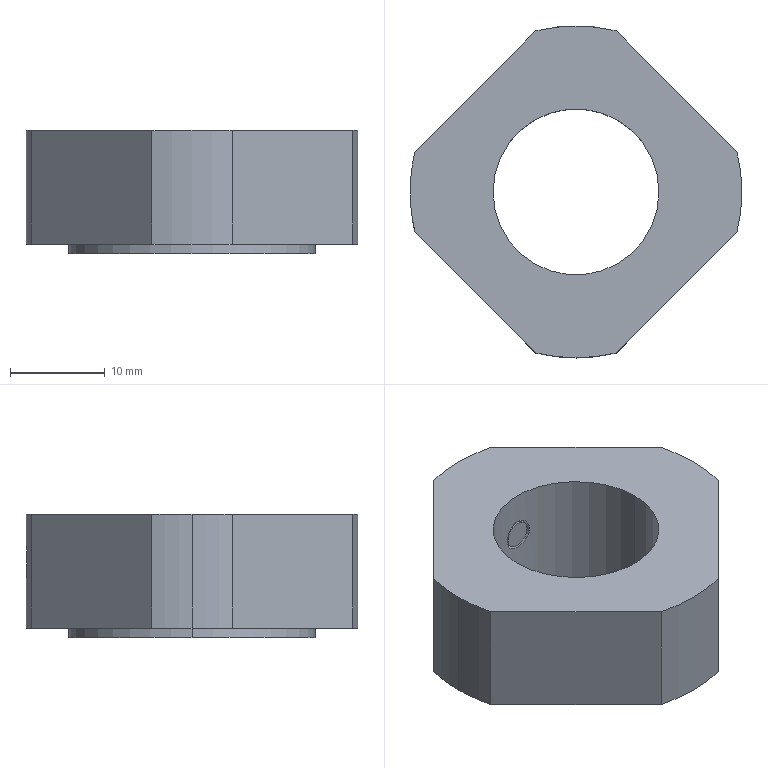Part | STEP file | Mirror BNG20 | 3 solids | 46 faces | box 35 x 35 x 13 mm | volume 7455 mm3 | plane 23 | cylinder 15 | cone 8 | commonest cylinder face diameters 35 x5 3 x2 3.3 x2 4 x2 17.5 x2 26 x2
STEP:
#1=CARTESIAN_POINT('',(-1.65,8.593,-5.));
#2=VERTEX_POINT('',#1);
#3=CARTESIAN_POINT('',(1.65,8.593,-5.));
#4=VERTEX_POINT('',#3);
#5=CARTESIAN_POINT('',(-1.65,8.593,-5.));
#6=CARTESIAN_POINT('',(-1.65,8.593,-5.109));
#7=CARTESIAN_POINT('',(-1.639,8.595,-5.217));
#8=CARTESIAN_POINT('',(-1.597,8.603,-5.428));
#9=CARTESIAN_POINT('',(-1.565,8.609,-5.533));
#10=CARTESIAN_POINT('',(-1.482,8.624,-5.733));
#11=CARTESIAN_POINT('',(-1.432,8.632,-5.827));
#12=CARTESIAN_POINT('',(-1.312,8.651,-6.006));
#13=CARTESIAN_POINT('',(-1.242,8.662,-6.091));
#14=CARTESIAN_POINT('',(-1.015,8.692,-6.319));
#15=CARTESIAN_POINT('',(-0.8309,8.713,-6.442));
#16=CARTESIAN_POINT('',(-0.4339,8.741,-6.606));
#17=CARTESIAN_POINT('',(-0.2164,8.75,-6.65));
#18=CARTESIAN_POINT('',(0.1073,8.75,-6.65));
#19=CARTESIAN_POINT('',(0.2169,8.748,-6.639));
#20=CARTESIAN_POINT('',(0.4287,8.74,-6.597));
#21=CARTESIAN_POINT('',(0.5317,8.734,-6.566));
#22=CARTESIAN_POINT('',(0.8318,8.713,-6.441));
#23=CARTESIAN_POINT('',(1.013,8.693,-6.32));
#24=CARTESIAN_POINT('',(1.244,8.662,-6.09));
#25=CARTESIAN_POINT('',(1.312,8.651,-6.007));
#26=CARTESIAN_POINT('',(1.431,8.632,-5.828));
#27=CARTESIAN_POINT('',(1.483,8.624,-5.732));
#28=CARTESIAN_POINT('',(1.566,8.609,-5.532));
#29=CARTESIAN_POINT('',(1.597,8.603,-5.429));
#30=CARTESIAN_POINT('',(1.639,8.595,-5.217));
#31=CARTESIAN_POINT('',(1.65,8.593,-5.108));
#32=CARTESIAN_POINT('',(1.65,8.593,-5.));
#33=B_SPLINE_CURVE_WITH_KNOTS('',3,(#5,#6,#7,#8,#9,#10,#11,#12,#13,#14,#15,#16,#17,#18,#19,#20,#21,#22,#23,#24,#25,#26,#27,#28,#29,#30,#31,#32),.UNSPECIFIED.,.F.,.F.,(4,2,2,2,2,2,2,2,2,2,2,2,2,4),(0.,0.0003231,0.0006463,0.0009694,0.001293,0.001939,0.002585,0.002908,0.003231,0.003878,0.004201,0.004524,0.004847,0.00517),.UNSPECIFIED.);
#34=EDGE_CURVE('',#2,#4,#33,.T.);
#35=ORIENTED_EDGE('',*,*,#34,.T.);
#36=CARTESIAN_POINT('',(1.65,17.422,-5.));
#37=VERTEX_POINT('',#36);
#38=CARTESIAN_POINT('',(1.65,17.5,-5.));
#39=DIRECTION('',(0.,1.,0.));
#40=VECTOR('',#39,1000.);
#41=LINE('',#38,#40);
#42=EDGE_CURVE('',#4,#37,#41,.T.);
#43=ORIENTED_EDGE('',*,*,#42,.T.);
#44=CARTESIAN_POINT('',(-1.65,17.422,-5.));
#45=VERTEX_POINT('',#44);
#46=CARTESIAN_POINT('',(1.65,17.422,-5.));
#47=CARTESIAN_POINT('',(1.65,17.422,-5.215));
#48=CARTESIAN_POINT('',(1.607,17.426,-5.433));
#49=CARTESIAN_POINT('',(1.442,17.441,-5.83));
#50=CARTESIAN_POINT('',(1.32,17.451,-6.014));
#51=CARTESIAN_POINT('',(1.092,17.466,-6.242));
#52=CARTESIAN_POINT('',(1.007,17.471,-6.312));
#53=CARTESIAN_POINT('',(0.8275,17.481,-6.432));
#54=CARTESIAN_POINT('',(0.7328,17.485,-6.482));
#55=CARTESIAN_POINT('',(0.5332,17.492,-6.565));
#56=CARTESIAN_POINT('',(0.4283,17.495,-6.597));
#57=CARTESIAN_POINT('',(0.2174,17.499,-6.639));
#58=CARTESIAN_POINT('',(0.1103,17.5,-6.65));
#59=CARTESIAN_POINT('',(-0.1077,17.5,-6.65));
#60=CARTESIAN_POINT('',(-0.2151,17.499,-6.639));
#61=CARTESIAN_POINT('',(-0.4261,17.495,-6.598));
#62=CARTESIAN_POINT('',(-0.5308,17.492,-6.566));
#63=CARTESIAN_POINT('',(-0.7308,17.485,-6.483));
#64=CARTESIAN_POINT('',(-0.8255,17.481,-6.433));
#65=CARTESIAN_POINT('',(-1.005,17.471,-6.313));
#66=CARTESIAN_POINT('',(-1.09,17.466,-6.244));
#67=CARTESIAN_POINT('',(-1.318,17.451,-6.016));
#68=CARTESIAN_POINT('',(-1.441,17.441,-5.832));
#69=CARTESIAN_POINT('',(-1.606,17.426,-5.435));
#70=CARTESIAN_POINT('',(-1.65,17.422,-5.218));
#71=CARTESIAN_POINT('',(-1.65,17.422,-5.));
#72=B_SPLINE_CURVE_WITH_KNOTS('',3,(#46,#47,#48,#49,#50,#51,#52,#53,#54,#55,#56,#57,#58,#59,#60,#61,#62,#63,#64,#65,#66,#67,#68,#69,#70,#71),.UNSPECIFIED.,.F.,.F.,(4,2,2,2,2,2,2,2,2,2,2,2,4),(0.005162,0.005807,0.006452,0.006774,0.007097,0.007419,0.007742,0.008064,0.008387,0.008709,0.009032,0.009677,0.01032),.UNSPECIFIED.);
#73=EDGE_CURVE('',#37,#45,#72,.T.);
#74=ORIENTED_EDGE('',*,*,#73,.T.);
#75=CARTESIAN_POINT('',(-1.65,17.5,-5.));
#76=DIRECTION('',(0.,1.,0.));
#77=VECTOR('',#76,1000.);
#78=LINE('',#75,#77);
#79=EDGE_CURVE('',#2,#45,#78,.T.);
#80=ORIENTED_EDGE('',*,*,#79,.F.);
#81=EDGE_LOOP('',(#35,#43,#74,#80));
#82=FACE_OUTER_BOUND('',#81,.T.);
#83=CARTESIAN_POINT('',(0.,17.5,-5.));
#84=DIRECTION('',(0.,1.,0.));
#85=DIRECTION('',(-1.,0.,0.));
#86=AXIS2_PLACEMENT_3D('',#83,#84,#85);
#87=CYLINDRICAL_SURFACE('',#86,1.65);
#88=ADVANCED_FACE('',(#82),#87,.F.);
#89=ORIENTED_EDGE('',*,*,#34,.F.);
#90=CARTESIAN_POINT('',(1.65,8.593,-5.));
#91=CARTESIAN_POINT('',(1.65,8.593,-4.784));
#92=CARTESIAN_POINT('',(1.607,8.602,-4.567));
#93=CARTESIAN_POINT('',(1.442,8.631,-4.17));
#94=CARTESIAN_POINT('',(1.319,8.651,-3.986));
#95=CARTESIAN_POINT('',(1.091,8.682,-3.758));
#96=CARTESIAN_POINT('',(1.007,8.692,-3.688));
#97=CARTESIAN_POINT('',(0.8281,8.711,-3.569));
#98=CARTESIAN_POINT('',(0.7335,8.72,-3.518));
#99=CARTESIAN_POINT('',(0.4333,8.742,-3.393));
#100=CARTESIAN_POINT('',(0.2188,8.75,-3.35));
#101=CARTESIAN_POINT('',(-0.1081,8.75,-3.35));
#102=CARTESIAN_POINT('',(-0.2154,8.748,-3.361));
#103=CARTESIAN_POINT('',(-0.4268,8.74,-3.403));
#104=CARTESIAN_POINT('',(-0.5319,8.734,-3.434));
#105=CARTESIAN_POINT('',(-0.7313,8.72,-3.517));
#106=CARTESIAN_POINT('',(-0.826,8.711,-3.568));
#107=CARTESIAN_POINT('',(-1.006,8.692,-3.687));
#108=CARTESIAN_POINT('',(-1.09,8.682,-3.757));
#109=CARTESIAN_POINT('',(-1.318,8.652,-3.984));
#110=CARTESIAN_POINT('',(-1.441,8.631,-4.168));
#111=CARTESIAN_POINT('',(-1.606,8.602,-4.565));
#112=CARTESIAN_POINT('',(-1.65,8.593,-4.781));
#113=CARTESIAN_POINT('',(-1.65,8.593,-5.));
#114=B_SPLINE_CURVE_WITH_KNOTS('',3,(#90,#91,#92,#93,#94,#95,#96,#97,#98,#99,#100,#101,#102,#103,#104,#105,#106,#107,#108,#109,#110,#111,#112,#113),.UNSPECIFIED.,.F.,.F.,(4,2,2,2,2,2,2,2,2,2,2,4),(0.00517,0.005816,0.006462,0.006786,0.007109,0.007755,0.008078,0.008401,0.008724,0.009047,0.009693,0.01034),.UNSPECIFIED.);
#115=EDGE_CURVE('',#4,#2,#114,.T.);
#116=ORIENTED_EDGE('',*,*,#115,.F.);
#117=EDGE_LOOP('',(#89,#116));
#118=FACE_BOUND('',#117,.T.);
#119=CARTESIAN_POINT('',(-8.75,0.,-13.));
#120=VERTEX_POINT('',#119);
#121=CARTESIAN_POINT('',(8.75,0.,-13.));
#122=VERTEX_POINT('',#121);
#123=CARTESIAN_POINT('',(0.,0.,-13.));
#124=DIRECTION('',(0.,0.,-1.));
#125=DIRECTION('',(-1.,0.,0.));
#126=AXIS2_PLACEMENT_3D('',#123,#124,#125);
#127=CIRCLE('',#126,8.75);
#128=EDGE_CURVE('',#120,#122,#127,.T.);
#129=ORIENTED_EDGE('',*,*,#128,.T.);
#130=CARTESIAN_POINT('',(8.75,0.,0.));
#131=VERTEX_POINT('',#130);
#132=CARTESIAN_POINT('',(8.75,0.,0.));
#133=DIRECTION('',(0.,0.,1.));
#134=VECTOR('',#133,1000.);
#135=LINE('',#132,#134);
#136=EDGE_CURVE('',#122,#131,#135,.T.);
#137=ORIENTED_EDGE('',*,*,#136,.T.);
#138=CARTESIAN_POINT('',(-8.75,0.,0.));
#139=VERTEX_POINT('',#138);
#140=CARTESIAN_POINT('',(0.,0.,0.));
#141=DIRECTION('',(0.,0.,-1.));
#142=DIRECTION('',(-1.,0.,0.));
#143=AXIS2_PLACEMENT_3D('',#140,#141,#142);
#144=CIRCLE('',#143,8.75);
#145=EDGE_CURVE('',#139,#131,#144,.T.);
#146=ORIENTED_EDGE('',*,*,#145,.F.);
#147=CARTESIAN_POINT('',(-8.75,0.,0.));
#148=DIRECTION('',(0.,0.,1.));
#149=VECTOR('',#148,1000.);
#150=LINE('',#147,#149);
#151=EDGE_CURVE('',#120,#139,#150,.T.);
#152=ORIENTED_EDGE('',*,*,#151,.F.);
#153=EDGE_LOOP('',(#129,#137,#146,#152));
#154=FACE_OUTER_BOUND('',#153,.T.);
#155=CARTESIAN_POINT('',(0.,0.,0.));
#156=DIRECTION('',(0.,0.,1.));
#157=DIRECTION('',(-1.,0.,0.));
#158=AXIS2_PLACEMENT_3D('',#155,#156,#157);
#159=CYLINDRICAL_SURFACE('',#158,8.75);
#160=ADVANCED_FACE('',(#118,#154),#159,.F.);
#161=CARTESIAN_POINT('',(13.,0.,-13.));
#162=VERTEX_POINT('',#161);
#163=CARTESIAN_POINT('',(-13.,0.,-13.));
#164=VERTEX_POINT('',#163);
#165=CARTESIAN_POINT('',(0.,0.,-13.));
#166=DIRECTION('',(0.,0.,-1.));
#167=DIRECTION('',(-1.,0.,0.));
#168=AXIS2_PLACEMENT_3D('',#165,#166,#167);
#169=CIRCLE('',#168,13.);
#170=EDGE_CURVE('',#162,#164,#169,.T.);
#171=ORIENTED_EDGE('',*,*,#170,.F.);
#172=CARTESIAN_POINT('',(13.,0.,-12.));
#173=VERTEX_POINT('',#172);
#174=CARTESIAN_POINT('',(13.,0.,0.));
#175=DIRECTION('',(0.,0.,1.));
#176=VECTOR('',#175,1000.);
#177=LINE('',#174,#176);
#178=EDGE_CURVE('',#162,#173,#177,.T.);
#179=ORIENTED_EDGE('',*,*,#178,.T.);
#180=CARTESIAN_POINT('',(-13.,0.,-12.));
#181=VERTEX_POINT('',#180);
#182=CARTESIAN_POINT('',(0.,0.,-12.));
#183=DIRECTION('',(0.,0.,-1.));
#184=DIRECTION('',(-1.,0.,0.));
#185=AXIS2_PLACEMENT_3D('',#182,#183,#184);
#186=CIRCLE('',#185,13.);
#187=EDGE_CURVE('',#173,#181,#186,.T.);
#188=ORIENTED_EDGE('',*,*,#187,.T.);
#189=CARTESIAN_POINT('',(-13.,0.,0.));
#190=DIRECTION('',(0.,0.,1.));
#191=VECTOR('',#190,1000.);
#192=LINE('',#189,#191);
#193=EDGE_CURVE('',#164,#181,#192,.T.);
#194=ORIENTED_EDGE('',*,*,#193,.F.);
#195=EDGE_LOOP('',(#171,#179,#188,#194));
#196=FACE_OUTER_BOUND('',#195,.T.);
#197=CARTESIAN_POINT('',(0.,0.,0.));
#198=DIRECTION('',(0.,0.,1.));
#199=DIRECTION('',(-1.,0.,0.));
#200=AXIS2_PLACEMENT_3D('',#197,#198,#199);
#201=CYLINDRICAL_SURFACE('',#200,13.);
#202=ADVANCED_FACE('',(#196),#201,.T.);
#203=CARTESIAN_POINT('',(-17.5,0.,-12.));
#204=VERTEX_POINT('',#203);
#205=CARTESIAN_POINT('',(-16.98,4.233,-12.));
#206=VERTEX_POINT('',#205);
#207=CARTESIAN_POINT('',(0.,0.,-12.));
#208=DIRECTION('',(0.,0.,-1.));
#209=DIRECTION('',(-1.,0.,0.));
#210=AXIS2_PLACEMENT_3D('',#207,#208,#209);
#211=CIRCLE('',#210,17.5);
#212=EDGE_CURVE('',#204,#206,#211,.T.);
#213=ORIENTED_EDGE('',*,*,#212,.F.);
#214=CARTESIAN_POINT('',(-17.5,0.,0.));
#215=VERTEX_POINT('',#214);
#216=CARTESIAN_POINT('',(-17.5,0.,0.));
#217=DIRECTION('',(0.,0.,1.));
#218=VECTOR('',#217,1000.);
#219=LINE('',#216,#218);
#220=EDGE_CURVE('',#204,#215,#219,.T.);
#221=ORIENTED_EDGE('',*,*,#220,.T.);
#222=CARTESIAN_POINT('',(-16.98,4.233,0.));
#223=VERTEX_POINT('',#222);
#224=CARTESIAN_POINT('',(0.,0.,0.));
#225=DIRECTION('',(0.,0.,-1.));
#226=DIRECTION('',(-1.,0.,0.));
#227=AXIS2_PLACEMENT_3D('',#224,#225,#226);
#228=CIRCLE('',#227,17.5);
#229=EDGE_CURVE('',#215,#223,#228,.T.);
#230=ORIENTED_EDGE('',*,*,#229,.T.);
#231=CARTESIAN_POINT('',(-16.98,4.233,-13.));
#232=DIRECTION('',(0.,0.,1.));
#233=VECTOR('',#232,1000.);
#234=LINE('',#231,#233);
#235=EDGE_CURVE('',#206,#223,#234,.T.);
#236=ORIENTED_EDGE('',*,*,#235,.F.);
#237=EDGE_LOOP('',(#213,#221,#230,#236));
#238=FACE_OUTER_BOUND('',#237,.T.);
#239=CARTESIAN_POINT('',(0.,0.,0.));
#240=DIRECTION('',(0.,0.,1.));
#241=DIRECTION('',(-1.,0.,0.));
#242=AXIS2_PLACEMENT_3D('',#239,#240,#241);
#243=CYLINDRICAL_SURFACE('',#242,17.5);
#244=ADVANCED_FACE('',(#238),#243,.T.);
#245=ORIENTED_EDGE('',*,*,#145,.T.);
#246=CARTESIAN_POINT('',(0.,0.,0.));
#247=DIRECTION('',(0.,0.,-1.));
#248=DIRECTION('',(-1.,0.,0.));
#249=AXIS2_PLACEMENT_3D('',#246,#247,#248);
#250=CIRCLE('',#249,8.75);
#251=EDGE_CURVE('',#131,#139,#250,.T.);
#252=ORIENTED_EDGE('',*,*,#251,.T.);
#253=EDGE_LOOP('',(#245,#252));
#254=FACE_BOUND('',#253,.T.);
#255=CARTESIAN_POINT('',(4.233,16.98,0.));
#256=VERTEX_POINT('',#255);
#257=CARTESIAN_POINT('',(16.98,4.233,0.));
#258=VERTEX_POINT('',#257);
#259=CARTESIAN_POINT('',(4.233,16.98,0.));
#260=DIRECTION('',(0.7071,-0.7071,0.));
#261=VECTOR('',#260,1000.);
#262=LINE('',#259,#261);
#263=EDGE_CURVE('',#256,#258,#262,.T.);
#264=ORIENTED_EDGE('',*,*,#263,.F.);
#265=CARTESIAN_POINT('',(-4.233,16.98,0.));
#266=VERTEX_POINT('',#265);
#267=CARTESIAN_POINT('',(0.,0.,0.));
#268=DIRECTION('',(0.,0.,-1.));
#269=DIRECTION('',(-1.,0.,0.));
#270=AXIS2_PLACEMENT_3D('',#267,#268,#269);
#271=CIRCLE('',#270,17.5);
#272=EDGE_CURVE('',#266,#256,#271,.T.);
#273=ORIENTED_EDGE('',*,*,#272,.F.);
#274=CARTESIAN_POINT('',(-16.98,4.233,0.));
#275=DIRECTION('',(0.7071,0.7071,0.));
#276=VECTOR('',#275,1000.);
#277=LINE('',#274,#276);
#278=EDGE_CURVE('',#223,#266,#277,.T.);
#279=ORIENTED_EDGE('',*,*,#278,.F.);
#280=ORIENTED_EDGE('',*,*,#229,.F.);
#281=CARTESIAN_POINT('',(-16.98,-4.233,0.));
#282=VERTEX_POINT('',#281);
#283=CARTESIAN_POINT('',(0.,0.,0.));
#284=DIRECTION('',(0.,0.,-1.));
#285=DIRECTION('',(-1.,0.,0.));
#286=AXIS2_PLACEMENT_3D('',#283,#284,#285);
#287=CIRCLE('',#286,17.5);
#288=EDGE_CURVE('',#282,#215,#287,.T.);
#289=ORIENTED_EDGE('',*,*,#288,.F.);
#290=CARTESIAN_POINT('',(-4.233,-16.98,0.));
#291=VERTEX_POINT('',#290);
#292=CARTESIAN_POINT('',(-16.98,-4.233,0.));
#293=DIRECTION('',(-0.7071,0.7071,0.));
#294=VECTOR('',#293,1000.);
#295=LINE('',#292,#294);
#296=EDGE_CURVE('',#291,#282,#295,.T.);
#297=ORIENTED_EDGE('',*,*,#296,.F.);
#298=CARTESIAN_POINT('',(4.233,-16.98,0.));
#299=VERTEX_POINT('',#298);
#300=CARTESIAN_POINT('',(0.,0.,0.));
#301=DIRECTION('',(0.,0.,-1.));
#302=DIRECTION('',(-1.,0.,0.));
#303=AXIS2_PLACEMENT_3D('',#300,#301,#302);
#304=CIRCLE('',#303,17.5);
#305=EDGE_CURVE('',#299,#291,#304,.T.);
#306=ORIENTED_EDGE('',*,*,#305,.F.);
#307=CARTESIAN_POINT('',(16.98,-4.233,0.));
#308=VERTEX_POINT('',#307);
#309=CARTESIAN_POINT('',(16.98,-4.233,0.));
#310=DIRECTION('',(-0.7071,-0.7071,0.));
#311=VECTOR('',#310,1000.);
#312=LINE('',#309,#311);
#313=EDGE_CURVE('',#308,#299,#312,.T.);
#314=ORIENTED_EDGE('',*,*,#313,.F.);
#315=CARTESIAN_POINT('',(0.,0.,0.));
#316=DIRECTION('',(0.,0.,-1.));
#317=DIRECTION('',(-1.,0.,0.));
#318=AXIS2_PLACEMENT_3D('',#315,#316,#317);
#319=CIRCLE('',#318,17.5);
#320=EDGE_CURVE('',#258,#308,#319,.T.);
#321=ORIENTED_EDGE('',*,*,#320,.F.);
#322=EDGE_LOOP('',(#264,#273,#279,#280,#289,#297,#306,#314,#321));
#323=FACE_OUTER_BOUND('',#322,.T.);
#324=CARTESIAN_POINT('',(0.,0.,0.));
#325=DIRECTION('',(0.,0.,-1.));
#326=DIRECTION('',(1.,0.,0.));
#327=AXIS2_PLACEMENT_3D('',#324,#325,#326);
#328=PLANE('',#327);
#329=ADVANCED_FACE('',(#254,#323),#328,.F.);
#330=CARTESIAN_POINT('',(16.98,4.233,-12.));
#331=VERTEX_POINT('',#330);
#332=CARTESIAN_POINT('',(16.98,4.233,-13.));
#333=DIRECTION('',(0.,0.,1.));
#334=VECTOR('',#333,1000.);
#335=LINE('',#332,#334);
#336=EDGE_CURVE('',#331,#258,#335,.T.);
#337=ORIENTED_EDGE('',*,*,#336,.T.);
#338=ORIENTED_EDGE('',*,*,#320,.T.);
#339=CARTESIAN_POINT('',(16.98,-4.233,-12.));
#340=VERTEX_POINT('',#339);
#341=CARTESIAN_POINT('',(16.98,-4.233,-13.));
#342=DIRECTION('',(0.,0.,1.));
#343=VECTOR('',#342,1000.);
#344=LINE('',#341,#343);
#345=EDGE_CURVE('',#340,#308,#344,.T.);
#346=ORIENTED_EDGE('',*,*,#345,.F.);
#347=CARTESIAN_POINT('',(0.,0.,-12.));
#348=DIRECTION('',(0.,0.,-1.));
#349=DIRECTION('',(-1.,0.,0.));
#350=AXIS2_PLACEMENT_3D('',#347,#348,#349);
#351=CIRCLE('',#350,17.5);
#352=EDGE_CURVE('',#331,#340,#351,.T.);
#353=ORIENTED_EDGE('',*,*,#352,.F.);
#354=EDGE_LOOP('',(#337,#338,#346,#353));
#355=FACE_OUTER_BOUND('',#354,.T.);
#356=CARTESIAN_POINT('',(0.,0.,0.));
#357=DIRECTION('',(0.,0.,1.));
#358=DIRECTION('',(-1.,0.,0.));
#359=AXIS2_PLACEMENT_3D('',#356,#357,#358);
#360=CYLINDRICAL_SURFACE('',#359,17.5);
#361=ADVANCED_FACE('',(#355),#360,.T.);
#362=CARTESIAN_POINT('',(-1.65,17.422,-5.));
#363=CARTESIAN_POINT('',(-1.65,17.422,-4.891));
#364=CARTESIAN_POINT('',(-1.639,17.423,-4.784));
#365=CARTESIAN_POINT('',(-1.597,17.427,-4.573));
#366=CARTESIAN_POINT('',(-1.566,17.43,-4.468));
#367=CARTESIAN_POINT('',(-1.483,17.437,-4.268));
#368=CARTESIAN_POINT('',(-1.432,17.441,-4.173));
#369=CARTESIAN_POINT('',(-1.312,17.451,-3.994));
#370=CARTESIAN_POINT('',(-1.243,17.456,-3.909));
#371=CARTESIAN_POINT('',(-1.014,17.471,-3.681));
#372=CARTESIAN_POINT('',(-0.8303,17.481,-3.558));
#373=CARTESIAN_POINT('',(-0.4332,17.496,-3.393));
#374=CARTESIAN_POINT('',(-0.216,17.5,-3.35));
#375=CARTESIAN_POINT('',(0.1071,17.5,-3.35));
#376=CARTESIAN_POINT('',(0.2165,17.499,-3.361));
#377=CARTESIAN_POINT('',(0.4281,17.495,-3.403));
#378=CARTESIAN_POINT('',(0.531,17.492,-3.434));
#379=CARTESIAN_POINT('',(0.7309,17.485,-3.517));
#380=CARTESIAN_POINT('',(0.8274,17.481,-3.568));
#381=CARTESIAN_POINT('',(1.006,17.471,-3.688));
#382=CARTESIAN_POINT('',(1.089,17.466,-3.756));
#383=CARTESIAN_POINT('',(1.244,17.456,-3.91));
#384=CARTESIAN_POINT('',(1.312,17.451,-3.993));
#385=CARTESIAN_POINT('',(1.431,17.441,-4.172));
#386=CARTESIAN_POINT('',(1.483,17.437,-4.269));
#387=CARTESIAN_POINT('',(1.566,17.43,-4.468));
#388=CARTESIAN_POINT('',(1.597,17.427,-4.571));
#389=CARTESIAN_POINT('',(1.639,17.423,-4.783));
#390=CARTESIAN_POINT('',(1.65,17.422,-4.892));
#391=CARTESIAN_POINT('',(1.65,17.422,-5.));
#392=B_SPLINE_CURVE_WITH_KNOTS('',3,(#362,#363,#364,#365,#366,#367,#368,#369,#370,#371,#372,#373,#374,#375,#376,#377,#378,#379,#380,#381,#382,#383,#384,#385,#386,#387,#388,#389,#390,#391),.UNSPECIFIED.,.F.,.F.,(4,2,2,2,2,2,2,2,2,2,2,2,2,2,4),(0.,0.0003226,0.0006452,0.0009678,0.00129,0.001936,0.002581,0.002903,0.003226,0.003549,0.003871,0.004194,0.004516,0.004839,0.005162),.UNSPECIFIED.);
#393=EDGE_CURVE('',#45,#37,#392,.T.);
#394=ORIENTED_EDGE('',*,*,#393,.F.);
#395=ORIENTED_EDGE('',*,*,#73,.F.);
#396=EDGE_LOOP('',(#394,#395));
#397=FACE_BOUND('',#396,.T.);
#398=CARTESIAN_POINT('',(4.233,16.98,-12.));
#399=VERTEX_POINT('',#398);
#400=CARTESIAN_POINT('',(4.233,16.98,-13.));
#401=DIRECTION('',(0.,0.,1.));
#402=VECTOR('',#401,1000.);
#403=LINE('',#400,#402);
#404=EDGE_CURVE('',#399,#256,#403,.T.);
#405=ORIENTED_EDGE('',*,*,#404,.F.);
#406=CARTESIAN_POINT('',(-4.233,16.98,-12.));
#407=VERTEX_POINT('',#406);
#408=CARTESIAN_POINT('',(0.,0.,-12.));
#409=DIRECTION('',(0.,0.,-1.));
#410=DIRECTION('',(-1.,0.,0.));
#411=AXIS2_PLACEMENT_3D('',#408,#409,#410);
#412=CIRCLE('',#411,17.5);
#413=EDGE_CURVE('',#407,#399,#412,.T.);
#414=ORIENTED_EDGE('',*,*,#413,.F.);
#415=CARTESIAN_POINT('',(-4.233,16.98,-13.));
#416=DIRECTION('',(0.,0.,1.));
#417=VECTOR('',#416,1000.);
#418=LINE('',#415,#417);
#419=EDGE_CURVE('',#407,#266,#418,.T.);
#420=ORIENTED_EDGE('',*,*,#419,.T.);
#421=ORIENTED_EDGE('',*,*,#272,.T.);
#422=EDGE_LOOP('',(#405,#414,#420,#421));
#423=FACE_OUTER_BOUND('',#422,.T.);
#424=CARTESIAN_POINT('',(0.,0.,0.));
#425=DIRECTION('',(0.,0.,1.));
#426=DIRECTION('',(-1.,0.,0.));
#427=AXIS2_PLACEMENT_3D('',#424,#425,#426);
#428=CYLINDRICAL_SURFACE('',#427,17.5);
#429=ADVANCED_FACE('',(#397,#423),#428,.T.);
#430=CARTESIAN_POINT('',(0.,0.,-12.));
#431=DIRECTION('',(0.,0.,-1.));
#432=DIRECTION('',(-1.,0.,0.));
#433=AXIS2_PLACEMENT_3D('',#430,#431,#432);
#434=CIRCLE('',#433,13.);
#435=EDGE_CURVE('',#181,#173,#434,.T.);
#436=ORIENTED_EDGE('',*,*,#435,.F.);
#437=ORIENTED_EDGE('',*,*,#187,.F.);
#438=EDGE_LOOP('',(#436,#437));
#439=FACE_BOUND('',#438,.T.);
#440=CARTESIAN_POINT('',(1.857,19.357,-12.));
#441=DIRECTION('',(0.7071,-0.7071,0.));
#442=VECTOR('',#441,1000.);
#443=LINE('',#440,#442);
#444=EDGE_CURVE('',#399,#331,#443,.T.);
#445=ORIENTED_EDGE('',*,*,#444,.T.);
#446=ORIENTED_EDGE('',*,*,#352,.T.);
#447=CARTESIAN_POINT('',(4.233,-16.98,-12.));
#448=VERTEX_POINT('',#447);
#449=CARTESIAN_POINT('',(19.357,-1.857,-12.));
#450=DIRECTION('',(-0.7071,-0.7071,0.));
#451=VECTOR('',#450,1000.);
#452=LINE('',#449,#451);
#453=EDGE_CURVE('',#340,#448,#452,.T.);
#454=ORIENTED_EDGE('',*,*,#453,.T.);
#455=CARTESIAN_POINT('',(-4.233,-16.98,-12.));
#456=VERTEX_POINT('',#455);
#457=CARTESIAN_POINT('',(0.,0.,-12.));
#458=DIRECTION('',(0.,0.,-1.));
#459=DIRECTION('',(-1.,0.,0.));
#460=AXIS2_PLACEMENT_3D('',#457,#458,#459);
#461=CIRCLE('',#460,17.5);
#462=EDGE_CURVE('',#448,#456,#461,.T.);
#463=ORIENTED_EDGE('',*,*,#462,.T.);
#464=CARTESIAN_POINT('',(-16.98,-4.233,-12.));
#465=VERTEX_POINT('',#464);
#466=CARTESIAN_POINT('',(-19.357,-1.857,-12.));
#467=DIRECTION('',(-0.7071,0.7071,0.));
#468=VECTOR('',#467,1000.);
#469=LINE('',#466,#468);
#470=EDGE_CURVE('',#456,#465,#469,.T.);
#471=ORIENTED_EDGE('',*,*,#470,.T.);
#472=CARTESIAN_POINT('',(0.,0.,-12.));
#473=DIRECTION('',(0.,0.,-1.));
#474=DIRECTION('',(-1.,0.,0.));
#475=AXIS2_PLACEMENT_3D('',#472,#473,#474);
#476=CIRCLE('',#475,17.5);
#477=EDGE_CURVE('',#465,#204,#476,.T.);
#478=ORIENTED_EDGE('',*,*,#477,.T.);
#479=ORIENTED_EDGE('',*,*,#212,.T.);
#480=CARTESIAN_POINT('',(-1.857,19.357,-12.));
#481=DIRECTION('',(0.7071,0.7071,0.));
#482=VECTOR('',#481,1000.);
#483=LINE('',#480,#482);
#484=EDGE_CURVE('',#206,#407,#483,.T.);
#485=ORIENTED_EDGE('',*,*,#484,.T.);
#486=ORIENTED_EDGE('',*,*,#413,.T.);
#487=EDGE_LOOP('',(#445,#446,#454,#463,#471,#478,#479,#485,#486));
#488=FACE_OUTER_BOUND('',#487,.T.);
#489=CARTESIAN_POINT('',(0.,17.5,-12.));
#490=DIRECTION('',(0.,0.,1.));
#491=DIRECTION('',(-1.,0.,0.));
#492=AXIS2_PLACEMENT_3D('',#489,#490,#491);
#493=PLANE('',#492);
#494=ADVANCED_FACE('',(#439,#488),#493,.F.);
#495=CARTESIAN_POINT('',(4.233,-16.98,-13.));
#496=DIRECTION('',(0.,0.,1.));
#497=VECTOR('',#496,1000.);
#498=LINE('',#495,#497);
#499=EDGE_CURVE('',#448,#299,#498,.T.);
#500=ORIENTED_EDGE('',*,*,#499,.T.);
#501=ORIENTED_EDGE('',*,*,#305,.T.);
#502=CARTESIAN_POINT('',(-4.233,-16.98,-13.));
#503=DIRECTION('',(0.,0.,1.));
#504=VECTOR('',#503,1000.);
#505=LINE('',#502,#504);
#506=EDGE_CURVE('',#456,#291,#505,.T.);
#507=ORIENTED_EDGE('',*,*,#506,.F.);
#508=ORIENTED_EDGE('',*,*,#462,.F.);
#509=EDGE_LOOP('',(#500,#501,#507,#508));
#510=FACE_OUTER_BOUND('',#509,.T.);
#511=CARTESIAN_POINT('',(0.,0.,0.));
#512=DIRECTION('',(0.,0.,1.));
#513=DIRECTION('',(-1.,0.,0.));
#514=AXIS2_PLACEMENT_3D('',#511,#512,#513);
#515=CYLINDRICAL_SURFACE('',#514,17.5);
#516=ADVANCED_FACE('',(#510),#515,.T.);
#517=ORIENTED_EDGE('',*,*,#220,.F.);
#518=ORIENTED_EDGE('',*,*,#477,.F.);
#519=CARTESIAN_POINT('',(-16.98,-4.233,-13.));
#520=DIRECTION('',(0.,0.,1.));
#521=VECTOR('',#520,1000.);
#522=LINE('',#519,#521);
#523=EDGE_CURVE('',#465,#282,#522,.T.);
#524=ORIENTED_EDGE('',*,*,#523,.T.);
#525=ORIENTED_EDGE('',*,*,#288,.T.);
#526=EDGE_LOOP('',(#517,#518,#524,#525));
#527=FACE_OUTER_BOUND('',#526,.T.);
#528=CARTESIAN_POINT('',(0.,0.,0.));
#529=DIRECTION('',(0.,0.,1.));
#530=DIRECTION('',(-1.,0.,0.));
#531=AXIS2_PLACEMENT_3D('',#528,#529,#530);
#532=CYLINDRICAL_SURFACE('',#531,17.5);
#533=ADVANCED_FACE('',(#527),#532,.T.);
#534=ORIENTED_EDGE('',*,*,#178,.F.);
#535=CARTESIAN_POINT('',(0.,0.,-13.));
#536=DIRECTION('',(0.,0.,-1.));
#537=DIRECTION('',(-1.,0.,0.));
#538=AXIS2_PLACEMENT_3D('',#535,#536,#537);
#539=CIRCLE('',#538,13.);
#540=EDGE_CURVE('',#164,#162,#539,.T.);
#541=ORIENTED_EDGE('',*,*,#540,.F.);
#542=ORIENTED_EDGE('',*,*,#193,.T.);
#543=ORIENTED_EDGE('',*,*,#435,.T.);
#544=EDGE_LOOP('',(#534,#541,#542,#543));
#545=FACE_OUTER_BOUND('',#544,.T.);
#546=CARTESIAN_POINT('',(0.,0.,0.));
#547=DIRECTION('',(0.,0.,1.));
#548=DIRECTION('',(-1.,0.,0.));
#549=AXIS2_PLACEMENT_3D('',#546,#547,#548);
#550=CYLINDRICAL_SURFACE('',#549,13.);
#551=ADVANCED_FACE('',(#545),#550,.T.);
#552=ORIENTED_EDGE('',*,*,#128,.F.);
#553=CARTESIAN_POINT('',(0.,0.,-13.));
#554=DIRECTION('',(0.,0.,-1.));
#555=DIRECTION('',(-1.,0.,0.));
#556=AXIS2_PLACEMENT_3D('',#553,#554,#555);
#557=CIRCLE('',#556,8.75);
#558=EDGE_CURVE('',#122,#120,#557,.T.);
#559=ORIENTED_EDGE('',*,*,#558,.F.);
#560=EDGE_LOOP('',(#552,#559));
#561=FACE_BOUND('',#560,.T.);
#562=ORIENTED_EDGE('',*,*,#540,.T.);
#563=ORIENTED_EDGE('',*,*,#170,.T.);
#564=EDGE_LOOP('',(#562,#563));
#565=FACE_OUTER_BOUND('',#564,.T.);
#566=CARTESIAN_POINT('',(0.,13.,-13.));
#567=DIRECTION('',(0.,0.,1.));
#568=DIRECTION('',(-1.,0.,0.));
#569=AXIS2_PLACEMENT_3D('',#566,#567,#568);
#570=PLANE('',#569);
#571=ADVANCED_FACE('',(#561,#565),#570,.F.);
#572=ORIENTED_EDGE('',*,*,#136,.F.);
#573=ORIENTED_EDGE('',*,*,#558,.T.);
#574=ORIENTED_EDGE('',*,*,#151,.T.);
#575=ORIENTED_EDGE('',*,*,#251,.F.);
#576=EDGE_LOOP('',(#572,#573,#574,#575));
#577=FACE_OUTER_BOUND('',#576,.T.);
#578=CARTESIAN_POINT('',(0.,0.,0.));
#579=DIRECTION('',(0.,0.,1.));
#580=DIRECTION('',(-1.,0.,0.));
#581=AXIS2_PLACEMENT_3D('',#578,#579,#580);
#582=CYLINDRICAL_SURFACE('',#581,8.75);
#583=ADVANCED_FACE('',(#577),#582,.F.);
#584=ORIENTED_EDGE('',*,*,#470,.F.);
#585=ORIENTED_EDGE('',*,*,#506,.T.);
#586=ORIENTED_EDGE('',*,*,#296,.T.);
#587=ORIENTED_EDGE('',*,*,#523,.F.);
#588=EDGE_LOOP('',(#584,#585,#586,#587));
#589=FACE_OUTER_BOUND('',#588,.T.);
#590=CARTESIAN_POINT('',(-16.98,-4.233,-13.));
#591=DIRECTION('',(-0.7071,-0.7071,0.));
#592=DIRECTION('',(0.7071,-0.7071,0.));
#593=AXIS2_PLACEMENT_3D('',#590,#591,#592);
#594=PLANE('',#593);
#595=ADVANCED_FACE('',(#589),#594,.T.);
#596=ORIENTED_EDGE('',*,*,#484,.F.);
#597=ORIENTED_EDGE('',*,*,#235,.T.);
#598=ORIENTED_EDGE('',*,*,#278,.T.);
#599=ORIENTED_EDGE('',*,*,#419,.F.);
#600=EDGE_LOOP('',(#596,#597,#598,#599));
#601=FACE_OUTER_BOUND('',#600,.T.);
#602=CARTESIAN_POINT('',(-16.98,4.233,-13.));
#603=DIRECTION('',(-0.7071,0.7071,0.));
#604=DIRECTION('',(-0.7071,-0.7071,0.));
#605=AXIS2_PLACEMENT_3D('',#602,#603,#604);
#606=PLANE('',#605);
#607=ADVANCED_FACE('',(#601),#606,.T.);
#608=ORIENTED_EDGE('',*,*,#453,.F.);
#609=ORIENTED_EDGE('',*,*,#345,.T.);
#610=ORIENTED_EDGE('',*,*,#313,.T.);
#611=ORIENTED_EDGE('',*,*,#499,.F.);
#612=EDGE_LOOP('',(#608,#609,#610,#611));
#613=FACE_OUTER_BOUND('',#612,.T.);
#614=CARTESIAN_POINT('',(16.98,-4.233,-13.));
#615=DIRECTION('',(0.7071,-0.7071,0.));
#616=DIRECTION('',(0.7071,0.7071,0.));
#617=AXIS2_PLACEMENT_3D('',#614,#615,#616);
#618=PLANE('',#617);
#619=ADVANCED_FACE('',(#613),#618,.T.);
#620=ORIENTED_EDGE('',*,*,#444,.F.);
#621=ORIENTED_EDGE('',*,*,#404,.T.);
#622=ORIENTED_EDGE('',*,*,#263,.T.);
#623=ORIENTED_EDGE('',*,*,#336,.F.);
#624=EDGE_LOOP('',(#620,#621,#622,#623));
#625=FACE_OUTER_BOUND('',#624,.T.);
#626=CARTESIAN_POINT('',(4.233,16.98,-13.));
#627=DIRECTION('',(0.7071,0.7071,0.));
#628=DIRECTION('',(-0.7071,0.7071,0.));
#629=AXIS2_PLACEMENT_3D('',#626,#627,#628);
#630=PLANE('',#629);
#631=ADVANCED_FACE('',(#625),#630,.T.);
#632=ORIENTED_EDGE('',*,*,#42,.F.);
#633=ORIENTED_EDGE('',*,*,#115,.T.);
#634=ORIENTED_EDGE('',*,*,#79,.T.);
#635=ORIENTED_EDGE('',*,*,#393,.T.);
#636=EDGE_LOOP('',(#632,#633,#634,#635));
#637=FACE_OUTER_BOUND('',#636,.T.);
#638=CARTESIAN_POINT('',(0.,17.5,-5.));
#639=DIRECTION('',(0.,1.,0.));
#640=DIRECTION('',(-1.,0.,0.));
#641=AXIS2_PLACEMENT_3D('',#638,#639,#640);
#642=CYLINDRICAL_SURFACE('',#641,1.65);
#643=ADVANCED_FACE('',(#637),#642,.F.);
#644=CLOSED_SHELL('',(#88,#160,#202,#244,#329,#361,#429,#494,#516,#533,#551,#571,#583,#595,#607,#619,#631,#643));
#645=MANIFOLD_SOLID_BREP('',#644);
#646=CARTESIAN_POINT('',(-1.25,13.5,-5.));
#647=VERTEX_POINT('',#646);
#648=CARTESIAN_POINT('',(1.25,13.5,-5.));
#649=VERTEX_POINT('',#648);
#650=CARTESIAN_POINT('',(0.,13.5,-5.));
#651=DIRECTION('',(0.,1.,0.));
#652=DIRECTION('',(1.,0.,0.));
#653=AXIS2_PLACEMENT_3D('',#650,#651,#652);
#654=CIRCLE('',#653,1.25);
#655=EDGE_CURVE('',#647,#649,#654,.T.);
#656=ORIENTED_EDGE('',*,*,#655,.T.);
#657=CARTESIAN_POINT('',(2.,14.25,-5.));
#658=VERTEX_POINT('',#657);
#659=CARTESIAN_POINT('',(2.,14.25,-5.));
#660=DIRECTION('',(0.7071,0.7071,0.));
#661=VECTOR('',#660,1000.);
#662=LINE('',#659,#661);
#663=EDGE_CURVE('',#649,#658,#662,.T.);
#664=ORIENTED_EDGE('',*,*,#663,.T.);
#665=CARTESIAN_POINT('',(0.,14.25,-3.));
#666=VERTEX_POINT('',#665);
#667=CARTESIAN_POINT('',(0.,14.25,-5.));
#668=DIRECTION('',(0.,1.,0.));
#669=DIRECTION('',(1.,0.,0.));
#670=AXIS2_PLACEMENT_3D('',#667,#668,#669);
#671=CIRCLE('',#670,2.);
#672=EDGE_CURVE('',#666,#658,#671,.T.);
#673=ORIENTED_EDGE('',*,*,#672,.F.);
#674=CARTESIAN_POINT('',(-2.,14.25,-5.));
#675=VERTEX_POINT('',#674);
#676=CARTESIAN_POINT('',(0.,14.25,-5.));
#677=DIRECTION('',(0.,1.,0.));
#678=DIRECTION('',(1.,0.,0.));
#679=AXIS2_PLACEMENT_3D('',#676,#677,#678);
#680=CIRCLE('',#679,2.);
#681=EDGE_CURVE('',#675,#666,#680,.T.);
#682=ORIENTED_EDGE('',*,*,#681,.F.);
#683=CARTESIAN_POINT('',(-2.,14.25,-5.));
#684=DIRECTION('',(-0.7071,0.7071,0.));
#685=VECTOR('',#684,1000.);
#686=LINE('',#683,#685);
#687=EDGE_CURVE('',#647,#675,#686,.T.);
#688=ORIENTED_EDGE('',*,*,#687,.F.);
#689=EDGE_LOOP('',(#656,#664,#673,#682,#688));
#690=FACE_OUTER_BOUND('',#689,.T.);
#691=CARTESIAN_POINT('',(0.,14.25,-5.));
#692=DIRECTION('',(0.,1.,0.));
#693=DIRECTION('',(-1.,0.,0.));
#694=AXIS2_PLACEMENT_3D('',#691,#692,#693);
#695=CONICAL_SURFACE('',#694,2.,0.7854);
#696=ADVANCED_FACE('',(#690),#695,.T.);
#697=CARTESIAN_POINT('',(0.,15.423,-5.));
#698=VERTEX_POINT('',#697);
#699=CARTESIAN_POINT('',(0.,16.,-4.));
#700=VERTEX_POINT('',#699);
#701=CARTESIAN_POINT('',(0.,15.423,-5.));
#702=DIRECTION('',(0.,0.5,0.866));
#703=VECTOR('',#702,1000.);
#704=LINE('',#701,#703);
#705=EDGE_CURVE('',#698,#700,#704,.T.);
#706=ORIENTED_EDGE('',*,*,#705,.F.);
#707=CARTESIAN_POINT('',(0.,16.,-6.));
#708=VERTEX_POINT('',#707);
#709=CARTESIAN_POINT('',(0.,15.423,-5.));
#710=DIRECTION('',(0.,0.5,-0.866));
#711=VECTOR('',#710,1000.);
#712=LINE('',#709,#711);
#713=EDGE_CURVE('',#698,#708,#712,.T.);
#714=ORIENTED_EDGE('',*,*,#713,.T.);
#715=CARTESIAN_POINT('',(-0.866,16.,-5.5));
#716=VERTEX_POINT('',#715);
#717=CARTESIAN_POINT('',(0.,16.,-5.));
#718=DIRECTION('',(0.,-1.,0.));
#719=DIRECTION('',(0.,0.,1.));
#720=AXIS2_PLACEMENT_3D('',#717,#718,#719);
#721=CIRCLE('',#720,1.);
#722=EDGE_CURVE('',#716,#708,#721,.T.);
#723=ORIENTED_EDGE('',*,*,#722,.F.);
#724=CARTESIAN_POINT('',(-0.866,16.,-4.5));
#725=VERTEX_POINT('',#724);
#726=CARTESIAN_POINT('',(0.,16.,-5.));
#727=DIRECTION('',(0.,-1.,0.));
#728=DIRECTION('',(0.,0.,1.));
#729=AXIS2_PLACEMENT_3D('',#726,#727,#728);
#730=CIRCLE('',#729,1.);
#731=EDGE_CURVE('',#725,#716,#730,.T.);
#732=ORIENTED_EDGE('',*,*,#731,.F.);
#733=CARTESIAN_POINT('',(0.,16.,-5.));
#734=DIRECTION('',(0.,-1.,0.));
#735=DIRECTION('',(0.,0.,1.));
#736=AXIS2_PLACEMENT_3D('',#733,#734,#735);
#737=CIRCLE('',#736,1.);
#738=EDGE_CURVE('',#700,#725,#737,.T.);
#739=ORIENTED_EDGE('',*,*,#738,.F.);
#740=EDGE_LOOP('',(#706,#714,#723,#732,#739));
#741=FACE_OUTER_BOUND('',#740,.T.);
#742=CARTESIAN_POINT('',(0.,1015.423,-5.));
#743=DIRECTION('',(0.,1.,0.));
#744=DIRECTION('',(0.,0.,1.));
#745=AXIS2_PLACEMENT_3D('',#742,#743,#744);
#746=CONICAL_SURFACE('',#745,1732.051,1.047);
#747=ADVANCED_FACE('',(#741),#746,.F.);
#748=ORIENTED_EDGE('',*,*,#672,.T.);
#749=CARTESIAN_POINT('',(0.,14.25,-7.));
#750=VERTEX_POINT('',#749);
#751=CARTESIAN_POINT('',(0.,14.25,-5.));
#752=DIRECTION('',(0.,1.,0.));
#753=DIRECTION('',(1.,0.,0.));
#754=AXIS2_PLACEMENT_3D('',#751,#752,#753);
#755=CIRCLE('',#754,2.);
#756=EDGE_CURVE('',#658,#750,#755,.T.);
#757=ORIENTED_EDGE('',*,*,#756,.T.);
#758=CARTESIAN_POINT('',(0.,17.5,-7.));
#759=VERTEX_POINT('',#758);
#760=CARTESIAN_POINT('',(0.,17.5,-7.));
#761=DIRECTION('',(0.,1.,0.));
#762=VECTOR('',#761,1000.);
#763=LINE('',#760,#762);
#764=EDGE_CURVE('',#750,#759,#763,.T.);
#765=ORIENTED_EDGE('',*,*,#764,.T.);
#766=CARTESIAN_POINT('',(0.,17.5,-3.));
#767=VERTEX_POINT('',#766);
#768=CARTESIAN_POINT('',(0.,17.5,-5.));
#769=DIRECTION('',(0.,-1.,0.));
#770=DIRECTION('',(0.,0.,1.));
#771=AXIS2_PLACEMENT_3D('',#768,#769,#770);
#772=CIRCLE('',#771,2.);
#773=EDGE_CURVE('',#759,#767,#772,.T.);
#774=ORIENTED_EDGE('',*,*,#773,.T.);
#775=CARTESIAN_POINT('',(0.,17.5,-3.));
#776=DIRECTION('',(0.,1.,0.));
#777=VECTOR('',#776,1000.);
#778=LINE('',#775,#777);
#779=EDGE_CURVE('',#666,#767,#778,.T.);
#780=ORIENTED_EDGE('',*,*,#779,.F.);
#781=EDGE_LOOP('',(#748,#757,#765,#774,#780));
#782=FACE_OUTER_BOUND('',#781,.T.);
#783=CARTESIAN_POINT('',(0.,17.5,-5.));
#784=DIRECTION('',(0.,1.,0.));
#785=DIRECTION('',(0.,0.,1.));
#786=AXIS2_PLACEMENT_3D('',#783,#784,#785);
#787=CYLINDRICAL_SURFACE('',#786,2.);
#788=ADVANCED_FACE('',(#782),#787,.T.);
#789=CARTESIAN_POINT('',(0.,17.5,-5.));
#790=DIRECTION('',(0.,-1.,0.));
#791=DIRECTION('',(0.,0.,1.));
#792=AXIS2_PLACEMENT_3D('',#789,#790,#791);
#793=CIRCLE('',#792,2.);
#794=EDGE_CURVE('',#767,#759,#793,.T.);
#795=ORIENTED_EDGE('',*,*,#794,.F.);
#796=ORIENTED_EDGE('',*,*,#773,.F.);
#797=EDGE_LOOP('',(#795,#796));
#798=FACE_OUTER_BOUND('',#797,.T.);
#799=CARTESIAN_POINT('',(1.155,17.5,-5.));
#800=VERTEX_POINT('',#799);
#801=CARTESIAN_POINT('',(0.5774,17.5,-4.));
#802=VERTEX_POINT('',#801);
#803=CARTESIAN_POINT('',(1.155,17.5,-5.));
#804=DIRECTION('',(-0.5,0.,0.866));
#805=VECTOR('',#804,1000.);
#806=LINE('',#803,#805);
#807=EDGE_CURVE('',#800,#802,#806,.T.);
#808=ORIENTED_EDGE('',*,*,#807,.T.);
#809=CARTESIAN_POINT('',(-0.5774,17.5,-4.));
#810=VERTEX_POINT('',#809);
#811=CARTESIAN_POINT('',(0.5774,17.5,-4.));
#812=DIRECTION('',(-1.,0.,0.));
#813=VECTOR('',#812,1000.);
#814=LINE('',#811,#813);
#815=EDGE_CURVE('',#802,#810,#814,.T.);
#816=ORIENTED_EDGE('',*,*,#815,.T.);
#817=CARTESIAN_POINT('',(-1.155,17.5,-5.));
#818=VERTEX_POINT('',#817);
#819=CARTESIAN_POINT('',(-0.5774,17.5,-4.));
#820=DIRECTION('',(-0.5,0.,-0.866));
#821=VECTOR('',#820,1000.);
#822=LINE('',#819,#821);
#823=EDGE_CURVE('',#810,#818,#822,.T.);
#824=ORIENTED_EDGE('',*,*,#823,.T.);
#825=CARTESIAN_POINT('',(-0.5774,17.5,-6.));
#826=VERTEX_POINT('',#825);
#827=CARTESIAN_POINT('',(-1.155,17.5,-5.));
#828=DIRECTION('',(0.5,0.,-0.866));
#829=VECTOR('',#828,1000.);
#830=LINE('',#827,#829);
#831=EDGE_CURVE('',#818,#826,#830,.T.);
#832=ORIENTED_EDGE('',*,*,#831,.T.);
#833=CARTESIAN_POINT('',(0.5774,17.5,-6.));
#834=VERTEX_POINT('',#833);
#835=CARTESIAN_POINT('',(-0.5774,17.5,-6.));
#836=DIRECTION('',(1.,0.,0.));
#837=VECTOR('',#836,1000.);
#838=LINE('',#835,#837);
#839=EDGE_CURVE('',#826,#834,#838,.T.);
#840=ORIENTED_EDGE('',*,*,#839,.T.);
#841=CARTESIAN_POINT('',(0.5774,17.5,-6.));
#842=DIRECTION('',(0.5,0.,0.866));
#843=VECTOR('',#842,1000.);
#844=LINE('',#841,#843);
#845=EDGE_CURVE('',#834,#800,#844,.T.);
#846=ORIENTED_EDGE('',*,*,#845,.T.);
#847=EDGE_LOOP('',(#808,#816,#824,#832,#840,#846));
#848=FACE_BOUND('',#847,.T.);
#849=CARTESIAN_POINT('',(0.,17.5,-5.));
#850=DIRECTION('',(0.,-1.,0.));
#851=DIRECTION('',(0.,0.,-1.));
#852=AXIS2_PLACEMENT_3D('',#849,#850,#851);
#853=PLANE('',#852);
#854=ADVANCED_FACE('',(#798,#848),#853,.F.);
#855=ORIENTED_EDGE('',*,*,#764,.F.);
#856=CARTESIAN_POINT('',(0.,14.25,-5.));
#857=DIRECTION('',(0.,1.,0.));
#858=DIRECTION('',(1.,0.,0.));
#859=AXIS2_PLACEMENT_3D('',#856,#857,#858);
#860=CIRCLE('',#859,2.);
#861=EDGE_CURVE('',#750,#675,#860,.T.);
#862=ORIENTED_EDGE('',*,*,#861,.T.);
#863=ORIENTED_EDGE('',*,*,#681,.T.);
#864=ORIENTED_EDGE('',*,*,#779,.T.);
#865=ORIENTED_EDGE('',*,*,#794,.T.);
#866=EDGE_LOOP('',(#855,#862,#863,#864,#865));
#867=FACE_OUTER_BOUND('',#866,.T.);
#868=CARTESIAN_POINT('',(0.,17.5,-5.));
#869=DIRECTION('',(0.,1.,0.));
#870=DIRECTION('',(0.,0.,1.));
#871=AXIS2_PLACEMENT_3D('',#868,#869,#870);
#872=CYLINDRICAL_SURFACE('',#871,2.);
#873=ADVANCED_FACE('',(#867),#872,.T.);
#874=CARTESIAN_POINT('',(0.5774,16.,-6.));
#875=VERTEX_POINT('',#874);
#876=CARTESIAN_POINT('',(0.866,16.,-5.5));
#877=VERTEX_POINT('',#876);
#878=CARTESIAN_POINT('',(0.5774,16.,-6.));
#879=DIRECTION('',(0.5,0.,0.866));
#880=VECTOR('',#879,1000.);
#881=LINE('',#878,#880);
#882=EDGE_CURVE('',#875,#877,#881,.T.);
#883=ORIENTED_EDGE('',*,*,#882,.T.);
#884=CARTESIAN_POINT('',(1.155,16.,-5.));
#885=VERTEX_POINT('',#884);
#886=CARTESIAN_POINT('',(0.5774,16.,-6.));
#887=DIRECTION('',(0.5,0.,0.866));
#888=VECTOR('',#887,1000.);
#889=LINE('',#886,#888);
#890=EDGE_CURVE('',#877,#885,#889,.T.);
#891=ORIENTED_EDGE('',*,*,#890,.T.);
#892=CARTESIAN_POINT('',(1.155,16.,-5.));
#893=DIRECTION('',(0.,1.,0.));
#894=VECTOR('',#893,1000.);
#895=LINE('',#892,#894);
#896=EDGE_CURVE('',#885,#800,#895,.T.);
#897=ORIENTED_EDGE('',*,*,#896,.T.);
#898=ORIENTED_EDGE('',*,*,#845,.F.);
#899=CARTESIAN_POINT('',(0.5774,16.,-6.));
#900=DIRECTION('',(0.,1.,0.));
#901=VECTOR('',#900,1000.);
#902=LINE('',#899,#901);
#903=EDGE_CURVE('',#875,#834,#902,.T.);
#904=ORIENTED_EDGE('',*,*,#903,.F.);
#905=EDGE_LOOP('',(#883,#891,#897,#898,#904));
#906=FACE_OUTER_BOUND('',#905,.T.);
#907=CARTESIAN_POINT('',(0.5774,16.,-6.));
#908=DIRECTION('',(0.866,0.,-0.5));
#909=DIRECTION('',(0.5,0.,0.866));
#910=AXIS2_PLACEMENT_3D('',#907,#908,#909);
#911=PLANE('',#910);
#912=ADVANCED_FACE('',(#906),#911,.F.);
#913=CARTESIAN_POINT('',(-0.5774,16.,-6.));
#914=VERTEX_POINT('',#913);
#915=CARTESIAN_POINT('',(-0.5774,16.,-6.));
#916=DIRECTION('',(1.,0.,0.));
#917=VECTOR('',#916,1000.);
#918=LINE('',#915,#917);
#919=EDGE_CURVE('',#914,#708,#918,.T.);
#920=ORIENTED_EDGE('',*,*,#919,.T.);
#921=CARTESIAN_POINT('',(-0.5774,16.,-6.));
#922=DIRECTION('',(1.,0.,0.));
#923=VECTOR('',#922,1000.);
#924=LINE('',#921,#923);
#925=EDGE_CURVE('',#708,#875,#924,.T.);
#926=ORIENTED_EDGE('',*,*,#925,.T.);
#927=ORIENTED_EDGE('',*,*,#903,.T.);
#928=ORIENTED_EDGE('',*,*,#839,.F.);
#929=CARTESIAN_POINT('',(-0.5774,16.,-6.));
#930=DIRECTION('',(0.,1.,0.));
#931=VECTOR('',#930,1000.);
#932=LINE('',#929,#931);
#933=EDGE_CURVE('',#914,#826,#932,.T.);
#934=ORIENTED_EDGE('',*,*,#933,.F.);
#935=EDGE_LOOP('',(#920,#926,#927,#928,#934));
#936=FACE_OUTER_BOUND('',#935,.T.);
#937=CARTESIAN_POINT('',(-0.5774,16.,-6.));
#938=DIRECTION('',(0.,0.,-1.));
#939=DIRECTION('',(1.,0.,0.));
#940=AXIS2_PLACEMENT_3D('',#937,#938,#939);
#941=PLANE('',#940);
#942=ADVANCED_FACE('',(#936),#941,.F.);
#943=CARTESIAN_POINT('',(-1.155,16.,-5.));
#944=VERTEX_POINT('',#943);
#945=CARTESIAN_POINT('',(-1.155,16.,-5.));
#946=DIRECTION('',(0.5,0.,-0.866));
#947=VECTOR('',#946,1000.);
#948=LINE('',#945,#947);
#949=EDGE_CURVE('',#944,#716,#948,.T.);
#950=ORIENTED_EDGE('',*,*,#949,.T.);
#951=CARTESIAN_POINT('',(-1.155,16.,-5.));
#952=DIRECTION('',(0.5,0.,-0.866));
#953=VECTOR('',#952,1000.);
#954=LINE('',#951,#953);
#955=EDGE_CURVE('',#716,#914,#954,.T.);
#956=ORIENTED_EDGE('',*,*,#955,.T.);
#957=ORIENTED_EDGE('',*,*,#933,.T.);
#958=ORIENTED_EDGE('',*,*,#831,.F.);
#959=CARTESIAN_POINT('',(-1.155,16.,-5.));
#960=DIRECTION('',(0.,1.,0.));
#961=VECTOR('',#960,1000.);
#962=LINE('',#959,#961);
#963=EDGE_CURVE('',#944,#818,#962,.T.);
#964=ORIENTED_EDGE('',*,*,#963,.F.);
#965=EDGE_LOOP('',(#950,#956,#957,#958,#964));
#966=FACE_OUTER_BOUND('',#965,.T.);
#967=CARTESIAN_POINT('',(-1.155,16.,-5.));
#968=DIRECTION('',(-0.866,0.,-0.5));
#969=DIRECTION('',(0.5,0.,-0.866));
#970=AXIS2_PLACEMENT_3D('',#967,#968,#969);
#971=PLANE('',#970);
#972=ADVANCED_FACE('',(#966),#971,.F.);
#973=CARTESIAN_POINT('',(-0.5774,16.,-4.));
#974=VERTEX_POINT('',#973);
#975=CARTESIAN_POINT('',(-0.5774,16.,-4.));
#976=DIRECTION('',(-0.5,0.,-0.866));
#977=VECTOR('',#976,1000.);
#978=LINE('',#975,#977);
#979=EDGE_CURVE('',#974,#725,#978,.T.);
#980=ORIENTED_EDGE('',*,*,#979,.T.);
#981=CARTESIAN_POINT('',(-0.5774,16.,-4.));
#982=DIRECTION('',(-0.5,0.,-0.866));
#983=VECTOR('',#982,1000.);
#984=LINE('',#981,#983);
#985=EDGE_CURVE('',#725,#944,#984,.T.);
#986=ORIENTED_EDGE('',*,*,#985,.T.);
#987=ORIENTED_EDGE('',*,*,#963,.T.);
#988=ORIENTED_EDGE('',*,*,#823,.F.);
#989=CARTESIAN_POINT('',(-0.5774,16.,-4.));
#990=DIRECTION('',(0.,1.,0.));
#991=VECTOR('',#990,1000.);
#992=LINE('',#989,#991);
#993=EDGE_CURVE('',#974,#810,#992,.T.);
#994=ORIENTED_EDGE('',*,*,#993,.F.);
#995=EDGE_LOOP('',(#980,#986,#987,#988,#994));
#996=FACE_OUTER_BOUND('',#995,.T.);
#997=CARTESIAN_POINT('',(-0.5774,16.,-4.));
#998=DIRECTION('',(-0.866,0.,0.5));
#999=DIRECTION('',(-0.5,0.,-0.866));
#1000=AXIS2_PLACEMENT_3D('',#997,#998,#999);
#1001=PLANE('',#1000);
#1002=ADVANCED_FACE('',(#996),#1001,.F.);
#1003=CARTESIAN_POINT('',(0.5774,16.,-4.));
#1004=VERTEX_POINT('',#1003);
#1005=CARTESIAN_POINT('',(0.5774,16.,-4.));
#1006=DIRECTION('',(-1.,0.,0.));
#1007=VECTOR('',#1006,1000.);
#1008=LINE('',#1005,#1007);
#1009=EDGE_CURVE('',#1004,#700,#1008,.T.);
#1010=ORIENTED_EDGE('',*,*,#1009,.T.);
#1011=CARTESIAN_POINT('',(0.5774,16.,-4.));
#1012=DIRECTION('',(-1.,0.,0.));
#1013=VECTOR('',#1012,1000.);
#1014=LINE('',#1011,#1013);
#1015=EDGE_CURVE('',#700,#974,#1014,.T.);
#1016=ORIENTED_EDGE('',*,*,#1015,.T.);
#1017=ORIENTED_EDGE('',*,*,#993,.T.);
#1018=ORIENTED_EDGE('',*,*,#815,.F.);
#1019=CARTESIAN_POINT('',(0.5774,16.,-4.));
#1020=DIRECTION('',(0.,1.,0.));
#1021=VECTOR('',#1020,1000.);
#1022=LINE('',#1019,#1021);
#1023=EDGE_CURVE('',#1004,#802,#1022,.T.);
#1024=ORIENTED_EDGE('',*,*,#1023,.F.);
#1025=EDGE_LOOP('',(#1010,#1016,#1017,#1018,#1024));
#1026=FACE_OUTER_BOUND('',#1025,.T.);
#1027=CARTESIAN_POINT('',(0.5774,16.,-4.));
#1028=DIRECTION('',(0.,0.,1.));
#1029=DIRECTION('',(-1.,0.,0.));
#1030=AXIS2_PLACEMENT_3D('',#1027,#1028,#1029);
#1031=PLANE('',#1030);
#1032=ADVANCED_FACE('',(#1026),#1031,.F.);
#1033=CARTESIAN_POINT('',(0.866,16.,-4.5));
#1034=VERTEX_POINT('',#1033);
#1035=CARTESIAN_POINT('',(1.155,16.,-5.));
#1036=DIRECTION('',(-0.5,0.,0.866));
#1037=VECTOR('',#1036,1000.);
#1038=LINE('',#1035,#1037);
#1039=EDGE_CURVE('',#885,#1034,#1038,.T.);
#1040=ORIENTED_EDGE('',*,*,#1039,.T.);
#1041=CARTESIAN_POINT('',(1.155,16.,-5.));
#1042=DIRECTION('',(-0.5,0.,0.866));
#1043=VECTOR('',#1042,1000.);
#1044=LINE('',#1041,#1043);
#1045=EDGE_CURVE('',#1034,#1004,#1044,.T.);
#1046=ORIENTED_EDGE('',*,*,#1045,.T.);
#1047=ORIENTED_EDGE('',*,*,#1023,.T.);
#1048=ORIENTED_EDGE('',*,*,#807,.F.);
#1049=ORIENTED_EDGE('',*,*,#896,.F.);
#1050=EDGE_LOOP('',(#1040,#1046,#1047,#1048,#1049));
#1051=FACE_OUTER_BOUND('',#1050,.T.);
#1052=CARTESIAN_POINT('',(1.155,16.,-5.));
#1053=DIRECTION('',(0.866,0.,0.5));
#1054=DIRECTION('',(-0.5,0.,0.866));
#1055=AXIS2_PLACEMENT_3D('',#1052,#1053,#1054);
#1056=PLANE('',#1055);
#1057=ADVANCED_FACE('',(#1051),#1056,.F.);
#1058=ORIENTED_EDGE('',*,*,#955,.F.);
#1059=ORIENTED_EDGE('',*,*,#722,.T.);
#1060=ORIENTED_EDGE('',*,*,#919,.F.);
#1061=EDGE_LOOP('',(#1058,#1059,#1060));
#1062=FACE_OUTER_BOUND('',#1061,.T.);
#1063=CARTESIAN_POINT('',(0.,16.,-5.));
#1064=DIRECTION('',(0.,1.,0.));
#1065=DIRECTION('',(-1.,0.,0.));
#1066=AXIS2_PLACEMENT_3D('',#1063,#1064,#1065);
#1067=PLANE('',#1066);
#1068=ADVANCED_FACE('',(#1062),#1067,.T.);
#1069=ORIENTED_EDGE('',*,*,#925,.F.);
#1070=CARTESIAN_POINT('',(0.,16.,-5.));
#1071=DIRECTION('',(0.,-1.,0.));
#1072=DIRECTION('',(0.,0.,1.));
#1073=AXIS2_PLACEMENT_3D('',#1070,#1071,#1072);
#1074=CIRCLE('',#1073,1.);
#1075=EDGE_CURVE('',#708,#877,#1074,.T.);
#1076=ORIENTED_EDGE('',*,*,#1075,.T.);
#1077=ORIENTED_EDGE('',*,*,#882,.F.);
#1078=EDGE_LOOP('',(#1069,#1076,#1077));
#1079=FACE_OUTER_BOUND('',#1078,.T.);
#1080=CARTESIAN_POINT('',(0.,16.,-5.));
#1081=DIRECTION('',(0.,1.,0.));
#1082=DIRECTION('',(-1.,0.,0.));
#1083=AXIS2_PLACEMENT_3D('',#1080,#1081,#1082);
#1084=PLANE('',#1083);
#1085=ADVANCED_FACE('',(#1079),#1084,.T.);
#1086=ORIENTED_EDGE('',*,*,#890,.F.);
#1087=CARTESIAN_POINT('',(0.,16.,-5.));
#1088=DIRECTION('',(0.,-1.,0.));
#1089=DIRECTION('',(0.,0.,1.));
#1090=AXIS2_PLACEMENT_3D('',#1087,#1088,#1089);
#1091=CIRCLE('',#1090,1.);
#1092=EDGE_CURVE('',#877,#1034,#1091,.T.);
#1093=ORIENTED_EDGE('',*,*,#1092,.T.);
#1094=ORIENTED_EDGE('',*,*,#1039,.F.);
#1095=EDGE_LOOP('',(#1086,#1093,#1094));
#1096=FACE_OUTER_BOUND('',#1095,.T.);
#1097=CARTESIAN_POINT('',(0.,16.,-5.));
#1098=DIRECTION('',(0.,1.,0.));
#1099=DIRECTION('',(-1.,0.,0.));
#1100=AXIS2_PLACEMENT_3D('',#1097,#1098,#1099);
#1101=PLANE('',#1100);
#1102=ADVANCED_FACE('',(#1096),#1101,.T.);
#1103=ORIENTED_EDGE('',*,*,#1045,.F.);
#1104=CARTESIAN_POINT('',(0.,16.,-5.));
#1105=DIRECTION('',(0.,-1.,0.));
#1106=DIRECTION('',(0.,0.,1.));
#1107=AXIS2_PLACEMENT_3D('',#1104,#1105,#1106);
#1108=CIRCLE('',#1107,1.);
#1109=EDGE_CURVE('',#1034,#700,#1108,.T.);
#1110=ORIENTED_EDGE('',*,*,#1109,.T.);
#1111=ORIENTED_EDGE('',*,*,#1009,.F.);
#1112=EDGE_LOOP('',(#1103,#1110,#1111));
#1113=FACE_OUTER_BOUND('',#1112,.T.);
#1114=CARTESIAN_POINT('',(0.,16.,-5.));
#1115=DIRECTION('',(0.,1.,0.));
#1116=DIRECTION('',(-1.,0.,0.));
#1117=AXIS2_PLACEMENT_3D('',#1114,#1115,#1116);
#1118=PLANE('',#1117);
#1119=ADVANCED_FACE('',(#1113),#1118,.T.);
#1120=ORIENTED_EDGE('',*,*,#1015,.F.);
#1121=ORIENTED_EDGE('',*,*,#738,.T.);
#1122=ORIENTED_EDGE('',*,*,#979,.F.);
#1123=EDGE_LOOP('',(#1120,#1121,#1122));
#1124=FACE_OUTER_BOUND('',#1123,.T.);
#1125=CARTESIAN_POINT('',(0.,16.,-5.));
#1126=DIRECTION('',(0.,1.,0.));
#1127=DIRECTION('',(-1.,0.,0.));
#1128=AXIS2_PLACEMENT_3D('',#1125,#1126,#1127);
#1129=PLANE('',#1128);
#1130=ADVANCED_FACE('',(#1124),#1129,.T.);
#1131=ORIENTED_EDGE('',*,*,#985,.F.);
#1132=ORIENTED_EDGE('',*,*,#731,.T.);
#1133=ORIENTED_EDGE('',*,*,#949,.F.);
#1134=EDGE_LOOP('',(#1131,#1132,#1133));
#1135=FACE_OUTER_BOUND('',#1134,.T.);
#1136=CARTESIAN_POINT('',(0.,16.,-5.));
#1137=DIRECTION('',(0.,1.,0.));
#1138=DIRECTION('',(-1.,0.,0.));
#1139=AXIS2_PLACEMENT_3D('',#1136,#1137,#1138);
#1140=PLANE('',#1139);
#1141=ADVANCED_FACE('',(#1135),#1140,.T.);
#1142=ORIENTED_EDGE('',*,*,#713,.F.);
#1143=ORIENTED_EDGE('',*,*,#705,.T.);
#1144=ORIENTED_EDGE('',*,*,#1109,.F.);
#1145=ORIENTED_EDGE('',*,*,#1092,.F.);
#1146=ORIENTED_EDGE('',*,*,#1075,.F.);
#1147=EDGE_LOOP('',(#1142,#1143,#1144,#1145,#1146));
#1148=FACE_OUTER_BOUND('',#1147,.T.);
#1149=CARTESIAN_POINT('',(0.,1015.423,-5.));
#1150=DIRECTION('',(0.,1.,0.));
#1151=DIRECTION('',(0.,0.,1.));
#1152=AXIS2_PLACEMENT_3D('',#1149,#1150,#1151);
#1153=CONICAL_SURFACE('',#1152,1732.051,1.047);
#1154=ADVANCED_FACE('',(#1148),#1153,.F.);
#1155=ORIENTED_EDGE('',*,*,#663,.F.);
#1156=CARTESIAN_POINT('',(0.,13.5,-5.));
#1157=DIRECTION('',(0.,1.,0.));
#1158=DIRECTION('',(1.,0.,0.));
#1159=AXIS2_PLACEMENT_3D('',#1156,#1157,#1158);
#1160=CIRCLE('',#1159,1.25);
#1161=EDGE_CURVE('',#649,#647,#1160,.T.);
#1162=ORIENTED_EDGE('',*,*,#1161,.T.);
#1163=ORIENTED_EDGE('',*,*,#687,.T.);
#1164=ORIENTED_EDGE('',*,*,#861,.F.);
#1165=ORIENTED_EDGE('',*,*,#756,.F.);
#1166=EDGE_LOOP('',(#1155,#1162,#1163,#1164,#1165));
#1167=FACE_OUTER_BOUND('',#1166,.T.);
#1168=CARTESIAN_POINT('',(0.,14.25,-5.));
#1169=DIRECTION('',(0.,1.,0.));
#1170=DIRECTION('',(-1.,0.,0.));
#1171=AXIS2_PLACEMENT_3D('',#1168,#1169,#1170);
#1172=CONICAL_SURFACE('',#1171,2.,0.7854);
#1173=ADVANCED_FACE('',(#1167),#1172,.T.);
#1174=ORIENTED_EDGE('',*,*,#655,.F.);
#1175=ORIENTED_EDGE('',*,*,#1161,.F.);
#1176=EDGE_LOOP('',(#1174,#1175));
#1177=FACE_OUTER_BOUND('',#1176,.T.);
#1178=CARTESIAN_POINT('',(0.,13.5,-7.));
#1179=DIRECTION('',(0.,1.,0.));
#1180=DIRECTION('',(0.,0.,1.));
#1181=AXIS2_PLACEMENT_3D('',#1178,#1179,#1180);
#1182=PLANE('',#1181);
#1183=ADVANCED_FACE('',(#1177),#1182,.F.);
#1184=CLOSED_SHELL('',(#696,#747,#788,#854,#873,#912,#942,#972,#1002,#1032,#1057,#1068,#1085,#1102,#1119,#1130,#1141,#1154,#1173,#1183));
#1185=MANIFOLD_SOLID_BREP('',#1184);
#1186=CARTESIAN_POINT('',(0.,9.25,-6.4));
#1187=VERTEX_POINT('',#1186);
#1188=CARTESIAN_POINT('',(0.,9.25,-3.6));
#1189=VERTEX_POINT('',#1188);
#1190=CARTESIAN_POINT('',(0.,9.25,-5.));
#1191=DIRECTION('',(0.,-1.,0.));
#1192=DIRECTION('',(0.,0.,-1.));
#1193=AXIS2_PLACEMENT_3D('',#1190,#1191,#1192);
#1194=CIRCLE('',#1193,1.4);
#1195=EDGE_CURVE('',#1187,#1189,#1194,.T.);
#1196=ORIENTED_EDGE('',*,*,#1195,.T.);
#1197=CARTESIAN_POINT('',(0.,9.15,-3.5));
#1198=VERTEX_POINT('',#1197);
#1199=CARTESIAN_POINT('',(0.,9.25,-3.6));
#1200=DIRECTION('',(0.,-0.7071,0.7071));
#1201=VECTOR('',#1200,1000.);
#1202=LINE('',#1199,#1201);
#1203=EDGE_CURVE('',#1189,#1198,#1202,.T.);
#1204=ORIENTED_EDGE('',*,*,#1203,.T.);
#1205=CARTESIAN_POINT('',(0.,9.15,-6.5));
#1206=VERTEX_POINT('',#1205);
#1207=CARTESIAN_POINT('',(0.,9.15,-5.));
#1208=DIRECTION('',(0.,1.,0.));
#1209=DIRECTION('',(0.,0.,-1.));
#1210=AXIS2_PLACEMENT_3D('',#1207,#1208,#1209);
#1211=CIRCLE('',#1210,1.5);
#1212=EDGE_CURVE('',#1198,#1206,#1211,.T.);
#1213=ORIENTED_EDGE('',*,*,#1212,.T.);
#1214=CARTESIAN_POINT('',(0.,9.25,-6.4));
#1215=DIRECTION('',(0.,-0.7071,-0.7071));
#1216=VECTOR('',#1215,1000.);
#1217=LINE('',#1214,#1216);
#1218=EDGE_CURVE('',#1187,#1206,#1217,.T.);
#1219=ORIENTED_EDGE('',*,*,#1218,.F.);
#1220=EDGE_LOOP('',(#1196,#1204,#1213,#1219));
#1221=FACE_OUTER_BOUND('',#1220,.T.);
#1222=CARTESIAN_POINT('',(0.,9.25,-5.));
#1223=DIRECTION('',(0.,-1.,0.));
#1224=DIRECTION('',(0.,0.,-1.));
#1225=AXIS2_PLACEMENT_3D('',#1222,#1223,#1224);
#1226=CONICAL_SURFACE('',#1225,1.4,0.7854);
#1227=ADVANCED_FACE('',(#1221),#1226,.T.);
#1228=CARTESIAN_POINT('',(0.,8.75,-3.6));
#1229=VERTEX_POINT('',#1228);
#1230=CARTESIAN_POINT('',(0.,8.75,-6.4));
#1231=VERTEX_POINT('',#1230);
#1232=CARTESIAN_POINT('',(0.,8.75,-5.));
#1233=DIRECTION('',(0.,1.,0.));
#1234=DIRECTION('',(0.,0.,1.));
#1235=AXIS2_PLACEMENT_3D('',#1232,#1233,#1234);
#1236=CIRCLE('',#1235,1.4);
#1237=EDGE_CURVE('',#1229,#1231,#1236,.T.);
#1238=ORIENTED_EDGE('',*,*,#1237,.T.);
#1239=CARTESIAN_POINT('',(0.,8.85,-6.5));
#1240=VERTEX_POINT('',#1239);
#1241=CARTESIAN_POINT('',(0.,8.85,-6.5));
#1242=DIRECTION('',(0.,0.7071,-0.7071));
#1243=VECTOR('',#1242,1000.);
#1244=LINE('',#1241,#1243);
#1245=EDGE_CURVE('',#1231,#1240,#1244,.T.);
#1246=ORIENTED_EDGE('',*,*,#1245,.T.);
#1247=CARTESIAN_POINT('',(0.,8.85,-3.5));
#1248=VERTEX_POINT('',#1247);
#1249=CARTESIAN_POINT('',(0.,8.85,-5.));
#1250=DIRECTION('',(0.,-1.,0.));
#1251=DIRECTION('',(0.,0.,1.));
#1252=AXIS2_PLACEMENT_3D('',#1249,#1250,#1251);
#1253=CIRCLE('',#1252,1.5);
#1254=EDGE_CURVE('',#1240,#1248,#1253,.T.);
#1255=ORIENTED_EDGE('',*,*,#1254,.T.);
#1256=CARTESIAN_POINT('',(0.,8.85,-3.5));
#1257=DIRECTION('',(0.,0.7071,0.7071));
#1258=VECTOR('',#1257,1000.);
#1259=LINE('',#1256,#1258);
#1260=EDGE_CURVE('',#1229,#1248,#1259,.T.);
#1261=ORIENTED_EDGE('',*,*,#1260,.F.);
#1262=EDGE_LOOP('',(#1238,#1246,#1255,#1261));
#1263=FACE_OUTER_BOUND('',#1262,.T.);
#1264=CARTESIAN_POINT('',(0.,8.85,-5.));
#1265=DIRECTION('',(0.,1.,0.));
#1266=DIRECTION('',(0.,0.,1.));
#1267=AXIS2_PLACEMENT_3D('',#1264,#1265,#1266);
#1268=CONICAL_SURFACE('',#1267,1.5,0.7854);
#1269=ADVANCED_FACE('',(#1263),#1268,.T.);
#1270=ORIENTED_EDGE('',*,*,#1254,.F.);
#1271=CARTESIAN_POINT('',(0.,9.25,-6.5));
#1272=DIRECTION('',(0.,1.,0.));
#1273=VECTOR('',#1272,1000.);
#1274=LINE('',#1271,#1273);
#1275=EDGE_CURVE('',#1240,#1206,#1274,.T.);
#1276=ORIENTED_EDGE('',*,*,#1275,.T.);
#1277=ORIENTED_EDGE('',*,*,#1212,.F.);
#1278=CARTESIAN_POINT('',(0.,9.25,-3.5));
#1279=DIRECTION('',(0.,1.,0.));
#1280=VECTOR('',#1279,1000.);
#1281=LINE('',#1278,#1280);
#1282=EDGE_CURVE('',#1248,#1198,#1281,.T.);
#1283=ORIENTED_EDGE('',*,*,#1282,.F.);
#1284=EDGE_LOOP('',(#1270,#1276,#1277,#1283));
#1285=FACE_OUTER_BOUND('',#1284,.T.);
#1286=CARTESIAN_POINT('',(0.,9.25,-5.));
#1287=DIRECTION('',(0.,1.,0.));
#1288=DIRECTION('',(0.,0.,1.));
#1289=AXIS2_PLACEMENT_3D('',#1286,#1287,#1288);
#1290=CYLINDRICAL_SURFACE('',#1289,1.5);
#1291=ADVANCED_FACE('',(#1285),#1290,.T.);
#1292=ORIENTED_EDGE('',*,*,#1195,.F.);
#1293=CARTESIAN_POINT('',(0.,9.25,-5.));
#1294=DIRECTION('',(0.,-1.,0.));
#1295=DIRECTION('',(0.,0.,-1.));
#1296=AXIS2_PLACEMENT_3D('',#1293,#1294,#1295);
#1297=CIRCLE('',#1296,1.4);
#1298=EDGE_CURVE('',#1189,#1187,#1297,.T.);
#1299=ORIENTED_EDGE('',*,*,#1298,.F.);
#1300=EDGE_LOOP('',(#1292,#1299));
#1301=FACE_OUTER_BOUND('',#1300,.T.);
#1302=CARTESIAN_POINT('',(0.,9.25,-5.));
#1303=DIRECTION('',(0.,-1.,0.));
#1304=DIRECTION('',(0.,0.,-1.));
#1305=AXIS2_PLACEMENT_3D('',#1302,#1303,#1304);
#1306=PLANE('',#1305);
#1307=ADVANCED_FACE('',(#1301),#1306,.F.);
#1308=ORIENTED_EDGE('',*,*,#1275,.F.);
#1309=CARTESIAN_POINT('',(0.,8.85,-5.));
#1310=DIRECTION('',(0.,-1.,0.));
#1311=DIRECTION('',(0.,0.,1.));
#1312=AXIS2_PLACEMENT_3D('',#1309,#1310,#1311);
#1313=CIRCLE('',#1312,1.5);
#1314=EDGE_CURVE('',#1248,#1240,#1313,.T.);
#1315=ORIENTED_EDGE('',*,*,#1314,.F.);
#1316=ORIENTED_EDGE('',*,*,#1282,.T.);
#1317=CARTESIAN_POINT('',(0.,9.15,-5.));
#1318=DIRECTION('',(0.,1.,0.));
#1319=DIRECTION('',(0.,0.,-1.));
#1320=AXIS2_PLACEMENT_3D('',#1317,#1318,#1319);
#1321=CIRCLE('',#1320,1.5);
#1322=EDGE_CURVE('',#1206,#1198,#1321,.T.);
#1323=ORIENTED_EDGE('',*,*,#1322,.F.);
#1324=EDGE_LOOP('',(#1308,#1315,#1316,#1323));
#1325=FACE_OUTER_BOUND('',#1324,.T.);
#1326=CARTESIAN_POINT('',(0.,9.25,-5.));
#1327=DIRECTION('',(0.,1.,0.));
#1328=DIRECTION('',(0.,0.,1.));
#1329=AXIS2_PLACEMENT_3D('',#1326,#1327,#1328);
#1330=CYLINDRICAL_SURFACE('',#1329,1.5);
#1331=ADVANCED_FACE('',(#1325),#1330,.T.);
#1332=ORIENTED_EDGE('',*,*,#1237,.F.);
#1333=CARTESIAN_POINT('',(0.,8.75,-5.));
#1334=DIRECTION('',(0.,1.,0.));
#1335=DIRECTION('',(0.,0.,1.));
#1336=AXIS2_PLACEMENT_3D('',#1333,#1334,#1335);
#1337=CIRCLE('',#1336,1.4);
#1338=EDGE_CURVE('',#1231,#1229,#1337,.T.);
#1339=ORIENTED_EDGE('',*,*,#1338,.F.);
#1340=EDGE_LOOP('',(#1332,#1339));
#1341=FACE_OUTER_BOUND('',#1340,.T.);
#1342=CARTESIAN_POINT('',(0.,8.75,-6.5));
#1343=DIRECTION('',(0.,1.,0.));
#1344=DIRECTION('',(0.,0.,1.));
#1345=AXIS2_PLACEMENT_3D('',#1342,#1343,#1344);
#1346=PLANE('',#1345);
#1347=ADVANCED_FACE('',(#1341),#1346,.F.);
#1348=ORIENTED_EDGE('',*,*,#1245,.F.);
#1349=ORIENTED_EDGE('',*,*,#1338,.T.);
#1350=ORIENTED_EDGE('',*,*,#1260,.T.);
#1351=ORIENTED_EDGE('',*,*,#1314,.T.);
#1352=EDGE_LOOP('',(#1348,#1349,#1350,#1351));
#1353=FACE_OUTER_BOUND('',#1352,.T.);
#1354=CARTESIAN_POINT('',(0.,8.85,-5.));
#1355=DIRECTION('',(0.,1.,0.));
#1356=DIRECTION('',(0.,0.,1.));
#1357=AXIS2_PLACEMENT_3D('',#1354,#1355,#1356);
#1358=CONICAL_SURFACE('',#1357,1.5,0.7854);
#1359=ADVANCED_FACE('',(#1353),#1358,.T.);
#1360=ORIENTED_EDGE('',*,*,#1203,.F.);
#1361=ORIENTED_EDGE('',*,*,#1298,.T.);
#1362=ORIENTED_EDGE('',*,*,#1218,.T.);
#1363=ORIENTED_EDGE('',*,*,#1322,.T.);
#1364=EDGE_LOOP('',(#1360,#1361,#1362,#1363));
#1365=FACE_OUTER_BOUND('',#1364,.T.);
#1366=CARTESIAN_POINT('',(0.,9.25,-5.));
#1367=DIRECTION('',(0.,-1.,0.));
#1368=DIRECTION('',(0.,0.,-1.));
#1369=AXIS2_PLACEMENT_3D('',#1366,#1367,#1368);
#1370=CONICAL_SURFACE('',#1369,1.4,0.7854);
#1371=ADVANCED_FACE('',(#1365),#1370,.T.);
#1372=CLOSED_SHELL('',(#1227,#1269,#1291,#1307,#1331,#1347,#1359,#1371));
#1373=MANIFOLD_SOLID_BREP('',#1372);
#1374=CARTESIAN_POINT('',(0.,0.,0.));
#1375=DIRECTION('',(0.,0.,1.));
#1376=DIRECTION('',(1.,0.,0.));
#1377=AXIS2_PLACEMENT_3D('',#1374,#1375,#1376);
#1378=(LENGTH_UNIT()NAMED_UNIT(*)SI_UNIT(.MILLI.,.METRE.));
#1379=UNCERTAINTY_MEASURE_WITH_UNIT(LENGTH_MEASURE(0.00001),#1378,'','');
#1380=(NAMED_UNIT(*)PLANE_ANGLE_UNIT()SI_UNIT($,.RADIAN.));
#1381=(NAMED_UNIT(*)SI_UNIT($,.STERADIAN.)SOLID_ANGLE_UNIT());
#1382=(GEOMETRIC_REPRESENTATION_CONTEXT(3)GLOBAL_UNCERTAINTY_ASSIGNED_CONTEXT((#1379))GLOBAL_UNIT_ASSIGNED_CONTEXT((#1378,#1380,#1381))REPRESENTATION_CONTEXT('',''));
#1383=ADVANCED_BREP_SHAPE_REPRESENTATION('',(#645,#1185,#1373,#1377),#1382);